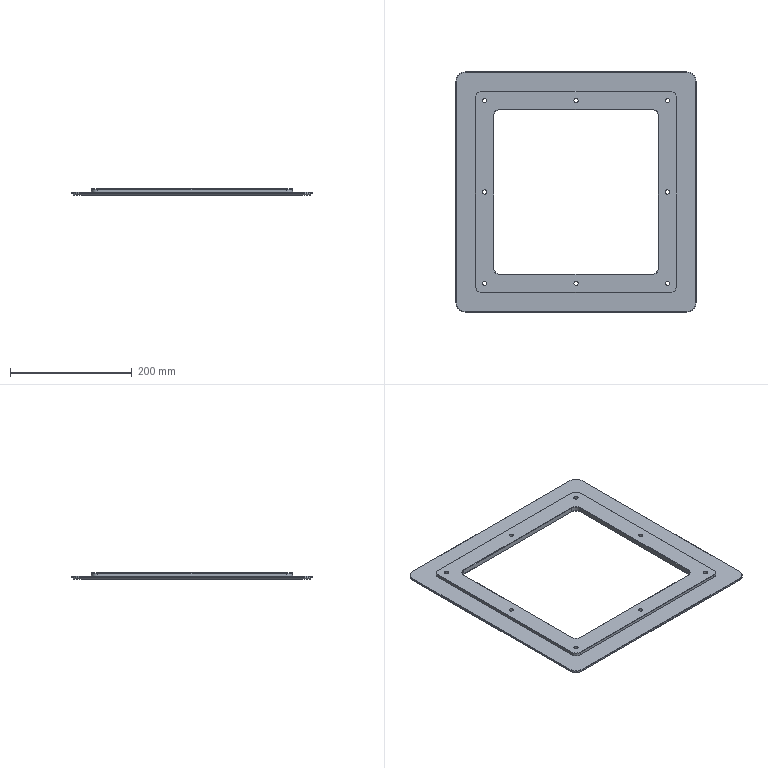CAM job | Mastercam | 3-axis milling, drilling
Tools:
tool_number,name,type,diameter_mm,corner_radius_mm,flutes,flute_length_mm,overall_length_mm,shoulder_length_mm,holder_diameter_mm,length_offset,diameter_offset,default_rpm,default_feed_mm_min,default_plunge_mm_min,coolant
7,10 Chamfer Mill,chamfer mill,10,0,4,25,75,30,50,7,7,3500,500,600,COOL_OFF
8,8 Flat End Mill,end mill,8,0,4,25,75,25,50,8,8,3500,1000,600,COOL_OFF
12,12 Flat End Mill,end mill,12,0,4,25,75,25,50,12,12,2000,800,600,COOL_OFF
14,20 Flat End Mill,end mill,20,0,4,25,75,25,50,14,14,1600,3000,600,COOL_OFF
24,63 Flat End Mill,end mill,63,0,4,25,75,25,50,24,24,500,300,600,COOL_OFF
Operations:
seq,operation,operation_type,tool_number,tool_name,tool_diameter_mm,spindle_rpm,feed_mm_min,plunge_mm_min,retract_mm_min,cycle_time_s,wcs,posted,nc_file
1,Contour (Ramp) - [WCS: Plane] - [Tplane: Plane],Contour,14,20 Flat End Mill,20,1600,3000,600,1200,44.612,Plane,yes,.nc
2,Contour (Ramp) - [WCS: Plane] - [Tplane: Plane],Contour,8,8 Flat End Mill,8,3500,1000,600,1200,163.081,Plane,yes,.nc
3,Pocket (Standard) - [WCS: Plane] - [Tplane: Plane],Pocket,14,20 Flat End Mill,20,1600,3200,1000,2000,1620.242,Plane,yes,.nc
4,Contour (Ramp) - [WCS: Plane] - [Tplane: Plane],Contour,14,20 Flat End Mill,20,1600,3000,600,1200,60.569,Plane,yes,.nc
5,Contour (Ramp) - [WCS: Plane] - [Tplane: Plane],Contour,14,20 Flat End Mill,20,1600,3000,600,1200,220.238,Plane,yes,.nc
6,Contour (Ramp) - [WCS: Plane] - [Tplane: Plane],Contour,14,20 Flat End Mill,20,2000,4000,600,1200,945.017,Plane,yes,.nc
7,Pocket (Standard) - [WCS: Plane] - [Tplane: Plane],Pocket,12,12 Flat End Mill,12,2000,800,600,1200,1809.325,Plane,yes,.nc
8,Contour (2D) - [WCS: Plane] - [Tplane: Plane],Contour,12,12 Flat End Mill,12,2000,800,600,1200,43.25,Plane,yes,.nc
9,Contour (2D) - [WCS: Plane] - [Tplane: Plane],Contour,12,12 Flat End Mill,12,2000,800,600,1200,240.893,Plane,yes,.nc
10,Contour (2D chamfer) - [WCS: Plane] - [Tplane: Plane],Contour,7,10 Chamfer Mill,10,3500,500,600,1200,631.531,Plane,yes,.nc
11,Drill/Counterbore - [WCS: Plane] - [Tplane: Plane],Drill,7,10 Chamfer Mill,10,3500,30,600,1200,31.028,Plane,yes,.nc
12,2D High Speed (2D Area Mill) - [WCS: Plane-1] - [Tplane: Plane-1],HighSpeed2D,14,20 Flat End Mill,20,1600,3000,600,1200,837.189,Plane-1,yes,.nc
13,2D High Speed (2D Area Mill) - [WCS: Plane-1] - [Tplane: Plane-1],HighSpeed2D,14,20 Flat End Mill,20,1600,3000,600,1200,1518.12,Plane-1,yes,.nc
14,Contour (Ramp) - [WCS: Plane-1] - [Tplane: Plane-1],Contour,14,20 Flat End Mill,20,1600,3000,600,1200,183.622,Plane-1,yes,.nc
15,Contour (2D) - [WCS: Plane-1] - [Tplane: Plane-1],Contour,24,63 Flat End Mill,63,1000,300,600,1200,291.188,Plane-1,yes,.nc
16,2D High Speed (2D Area Mill) - [WCS: Plane-1] - [Tplane: Plane-1],HighSpeed2D,12,12 Flat End Mill,12,2000,800,600,1200,450.174,Plane-1,yes,.nc
17,Contour (2D) - [WCS: Plane-1] - [Tplane: Plane-1],Contour,12,12 Flat End Mill,12,2000,800,600,1200,202.628,Plane-1,yes,.nc
18,Contour (2D chamfer) - [WCS: Plane-1] - [Tplane: Plane-1],Contour,7,10 Chamfer Mill,10,3500,500,600,1200,474.196,Plane-1,yes,.nc
19,Manual Entry (ou),ManualEntry,,,,0,0,0,0,0,Plane-1,yes,.nc
20,Contour (Ramp) - [WCS: Plane-1] - [Tplane: Plane-1],Contour,14,20 Flat End Mill,20,1600,3000,600,1200,679.535,Plane-1,yes,.nc
21,Contour (2D) - [WCS: Plane-1] - [Tplane: Plane-1],Contour,12,12 Flat End Mill,12,2000,800,600,1200,156.308,Plane-1,yes,.nc